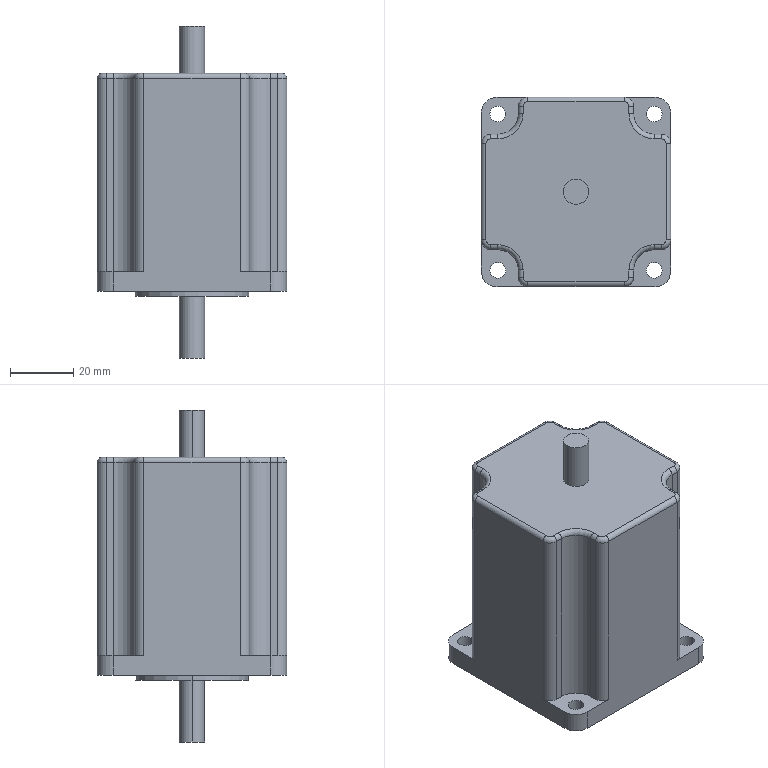Part | NX | features BREP 1 | 1 solid | 75 faces | box 60 x 60 x 105.1 mm | volume 217707 mm3 | cylinder 42 | plane 21 | torus 12 | commonest cylinder face diameters 3 x12 5 x8 6 x8 8 x4 10 x4 13 x4